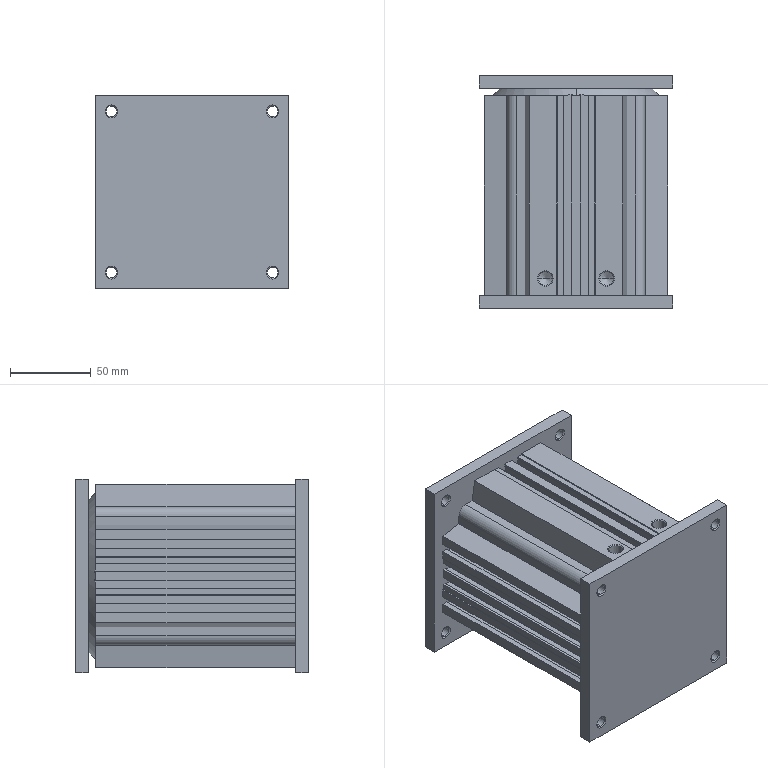Part | SolidWorks | features AEMSimFeature 1 | 2 solids | 301 faces | box 120 x 144.5 x 120 mm | volume 1424542 mm3 | plane 223 | cone 42 | cylinder 36 | commonest cylinder face diameters 6.647 x16 8.566 x4 12 x4 20 x4 40 x4 90 x4